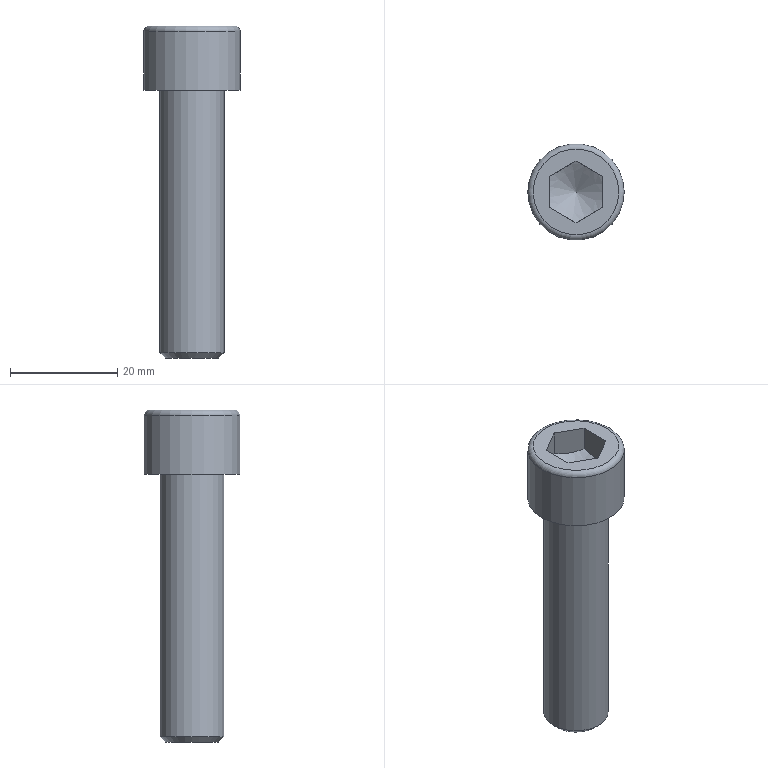Part | NX | features solid 2 | 1 solid | 14 faces | box 18 x 18 x 62 mm | volume 8162 mm3 | plane 9 | cylinder 2 | cone 2 | torus 1 | commonest cylinder face diameters 12 x1 18 x1
STEP:
#1=CARTESIAN_POINT('',(243.,-220.,-80.));
#2=VERTEX_POINT('',#1);
#3=CARTESIAN_POINT('',(235.,-220.,-80.));
#4=DIRECTION('',(0.,0.,1.));
#5=DIRECTION('',(1.,0.,0.));
#6=AXIS2_PLACEMENT_3D('',#3,#4,#5);
#7=CIRCLE('',#6,8.);
#8=EDGE_CURVE('',#2,#2,#7,.T.);
#9=ORIENTED_EDGE('',*,*,#8,.T.);
#10=EDGE_LOOP('',(#9));
#11=FACE_BOUND('',#10,.T.);
#12=CARTESIAN_POINT('',(240.,-222.887,-80.));
#13=VERTEX_POINT('',#12);
#14=CARTESIAN_POINT('',(235.,-225.774,-80.));
#15=VERTEX_POINT('',#14);
#16=CARTESIAN_POINT('',(240.,-222.887,-80.));
#17=DIRECTION('',(-0.866,-0.5,0.));
#18=VECTOR('',#17,1000.);
#19=LINE('',#16,#18);
#20=EDGE_CURVE('',#13,#15,#19,.T.);
#21=ORIENTED_EDGE('',*,*,#20,.T.);
#22=CARTESIAN_POINT('',(230.,-222.887,-80.));
#23=VERTEX_POINT('',#22);
#24=CARTESIAN_POINT('',(235.,-225.774,-80.));
#25=DIRECTION('',(-0.866,0.5,0.));
#26=VECTOR('',#25,1000.);
#27=LINE('',#24,#26);
#28=EDGE_CURVE('',#15,#23,#27,.T.);
#29=ORIENTED_EDGE('',*,*,#28,.T.);
#30=CARTESIAN_POINT('',(230.,-217.113,-80.));
#31=VERTEX_POINT('',#30);
#32=CARTESIAN_POINT('',(230.,-222.887,-80.));
#33=DIRECTION('',(0.,1.,0.));
#34=VECTOR('',#33,1000.);
#35=LINE('',#32,#34);
#36=EDGE_CURVE('',#23,#31,#35,.T.);
#37=ORIENTED_EDGE('',*,*,#36,.T.);
#38=CARTESIAN_POINT('',(235.,-214.226,-80.));
#39=VERTEX_POINT('',#38);
#40=CARTESIAN_POINT('',(230.,-217.113,-80.));
#41=DIRECTION('',(0.866,0.5,0.));
#42=VECTOR('',#41,1000.);
#43=LINE('',#40,#42);
#44=EDGE_CURVE('',#31,#39,#43,.T.);
#45=ORIENTED_EDGE('',*,*,#44,.T.);
#46=CARTESIAN_POINT('',(240.,-217.113,-80.));
#47=VERTEX_POINT('',#46);
#48=CARTESIAN_POINT('',(235.,-214.226,-80.));
#49=DIRECTION('',(0.866,-0.5,0.));
#50=VECTOR('',#49,1000.);
#51=LINE('',#48,#50);
#52=EDGE_CURVE('',#39,#47,#51,.T.);
#53=ORIENTED_EDGE('',*,*,#52,.T.);
#54=CARTESIAN_POINT('',(240.,-217.113,-80.));
#55=DIRECTION('',(0.,-1.,0.));
#56=VECTOR('',#55,1000.);
#57=LINE('',#54,#56);
#58=EDGE_CURVE('',#47,#13,#57,.T.);
#59=ORIENTED_EDGE('',*,*,#58,.T.);
#60=EDGE_LOOP('',(#21,#29,#37,#45,#53,#59));
#61=FACE_BOUND('',#60,.T.);
#62=CARTESIAN_POINT('',(235.,-220.,-80.));
#63=DIRECTION('',(0.,0.,1.));
#64=DIRECTION('',(1.,0.,0.));
#65=AXIS2_PLACEMENT_3D('',#62,#63,#64);
#66=PLANE('',#65);
#67=ADVANCED_FACE('',(#11,#61),#66,.T.);
#68=CARTESIAN_POINT('',(229.,-220.,-92.));
#69=VERTEX_POINT('',#68);
#70=CARTESIAN_POINT('',(235.,-220.,-92.));
#71=DIRECTION('',(0.,0.,-1.));
#72=DIRECTION('',(-1.,0.,0.));
#73=AXIS2_PLACEMENT_3D('',#70,#71,#72);
#74=CIRCLE('',#73,6.);
#75=EDGE_CURVE('',#69,#69,#74,.T.);
#76=ORIENTED_EDGE('',*,*,#75,.F.);
#77=EDGE_LOOP('',(#76));
#78=FACE_BOUND('',#77,.T.);
#79=CARTESIAN_POINT('',(244.,-220.,-92.));
#80=VERTEX_POINT('',#79);
#81=CARTESIAN_POINT('',(235.,-220.,-92.));
#82=DIRECTION('',(0.,0.,1.));
#83=DIRECTION('',(1.,0.,0.));
#84=AXIS2_PLACEMENT_3D('',#81,#82,#83);
#85=CIRCLE('',#84,9.);
#86=EDGE_CURVE('',#80,#80,#85,.T.);
#87=ORIENTED_EDGE('',*,*,#86,.F.);
#88=EDGE_LOOP('',(#87));
#89=FACE_BOUND('',#88,.T.);
#90=CARTESIAN_POINT('',(235.,-220.,-92.));
#91=DIRECTION('',(0.,0.,-1.));
#92=DIRECTION('',(-1.,0.,0.));
#93=AXIS2_PLACEMENT_3D('',#90,#91,#92);
#94=PLANE('',#93);
#95=ADVANCED_FACE('',(#78,#89),#94,.T.);
#96=CARTESIAN_POINT('',(244.,-220.,-81.));
#97=VERTEX_POINT('',#96);
#98=CARTESIAN_POINT('',(235.,-220.,-81.));
#99=DIRECTION('',(0.,0.,1.));
#100=DIRECTION('',(1.,0.,0.));
#101=AXIS2_PLACEMENT_3D('',#98,#99,#100);
#102=CIRCLE('',#101,9.);
#103=EDGE_CURVE('',#97,#97,#102,.F.);
#104=ORIENTED_EDGE('',*,*,#103,.T.);
#105=EDGE_LOOP('',(#104));
#106=FACE_BOUND('',#105,.T.);
#107=ORIENTED_EDGE('',*,*,#86,.T.);
#108=EDGE_LOOP('',(#107));
#109=FACE_BOUND('',#108,.T.);
#110=CARTESIAN_POINT('',(235.,-220.,-92.));
#111=DIRECTION('',(0.,0.,1.));
#112=DIRECTION('',(1.,0.,0.));
#113=AXIS2_PLACEMENT_3D('',#110,#111,#112);
#114=CYLINDRICAL_SURFACE('',#113,9.);
#115=ADVANCED_FACE('',(#106,#109),#114,.T.);
#116=CARTESIAN_POINT('',(235.,-225.774,-84.667));
#117=VERTEX_POINT('',#116);
#118=CARTESIAN_POINT('',(235.,-225.774,-80.));
#119=DIRECTION('',(0.,0.,-1.));
#120=VECTOR('',#119,1000.);
#121=LINE('',#118,#120);
#122=EDGE_CURVE('',#15,#117,#121,.T.);
#123=ORIENTED_EDGE('',*,*,#122,.F.);
#124=ORIENTED_EDGE('',*,*,#20,.F.);
#125=CARTESIAN_POINT('',(240.,-222.887,-84.667));
#126=VERTEX_POINT('',#125);
#127=CARTESIAN_POINT('',(240.,-222.887,-80.));
#128=DIRECTION('',(0.,0.,-1.));
#129=VECTOR('',#128,1000.);
#130=LINE('',#127,#129);
#131=EDGE_CURVE('',#13,#126,#130,.T.);
#132=ORIENTED_EDGE('',*,*,#131,.T.);
#133=CARTESIAN_POINT('',(235.,-225.774,-84.667));
#134=CARTESIAN_POINT('',(235.816,-225.302,-84.939));
#135=CARTESIAN_POINT('',(237.491,-224.335,-85.288));
#136=CARTESIAN_POINT('',(239.183,-223.359,-84.939));
#137=CARTESIAN_POINT('',(240.,-222.887,-84.667));
#138=B_SPLINE_CURVE_WITH_KNOTS('',3,(#133,#134,#135,#136,#137),.UNSPECIFIED.,.F.,.F.,(4,1,4),(0.000000238,0.002916,0.005831),.UNSPECIFIED.);
#139=EDGE_CURVE('',#117,#126,#138,.T.);
#140=ORIENTED_EDGE('',*,*,#139,.F.);
#141=EDGE_LOOP('',(#123,#124,#132,#140));
#142=FACE_BOUND('',#141,.T.);
#143=CARTESIAN_POINT('',(237.5,-224.33,-84.));
#144=DIRECTION('',(0.5,-0.866,0.));
#145=DIRECTION('',(0.866,0.5,0.));
#146=AXIS2_PLACEMENT_3D('',#143,#144,#145);
#147=PLANE('',#146);
#148=ADVANCED_FACE('',(#142),#147,.F.);
#149=ORIENTED_EDGE('',*,*,#131,.F.);
#150=ORIENTED_EDGE('',*,*,#58,.F.);
#151=CARTESIAN_POINT('',(240.,-217.113,-84.667));
#152=VERTEX_POINT('',#151);
#153=CARTESIAN_POINT('',(240.,-217.113,-80.));
#154=DIRECTION('',(0.,0.,-1.));
#155=VECTOR('',#154,1000.);
#156=LINE('',#153,#155);
#157=EDGE_CURVE('',#47,#152,#156,.T.);
#158=ORIENTED_EDGE('',*,*,#157,.T.);
#159=CARTESIAN_POINT('',(240.,-222.887,-84.667));
#160=CARTESIAN_POINT('',(240.,-221.948,-84.938));
#161=CARTESIAN_POINT('',(240.,-220.001,-85.29));
#162=CARTESIAN_POINT('',(240.,-218.046,-84.936));
#163=CARTESIAN_POINT('',(240.,-217.113,-84.667));
#164=B_SPLINE_CURVE_WITH_KNOTS('',3,(#159,#160,#161,#162,#163),.UNSPECIFIED.,.F.,.F.,(4,1,4),(0.005117,0.008037,0.01096),.UNSPECIFIED.);
#165=EDGE_CURVE('',#126,#152,#164,.T.);
#166=ORIENTED_EDGE('',*,*,#165,.F.);
#167=EDGE_LOOP('',(#149,#150,#158,#166));
#168=FACE_BOUND('',#167,.T.);
#169=CARTESIAN_POINT('',(240.,-220.,-84.));
#170=DIRECTION('',(1.,0.,0.));
#171=DIRECTION('',(0.,0.,-1.));
#172=AXIS2_PLACEMENT_3D('',#169,#170,#171);
#173=PLANE('',#172);
#174=ADVANCED_FACE('',(#168),#173,.F.);
#175=ORIENTED_EDGE('',*,*,#157,.F.);
#176=ORIENTED_EDGE('',*,*,#52,.F.);
#177=CARTESIAN_POINT('',(235.,-214.226,-84.667));
#178=VERTEX_POINT('',#177);
#179=CARTESIAN_POINT('',(235.,-214.226,-80.));
#180=DIRECTION('',(0.,0.,-1.));
#181=VECTOR('',#180,1000.);
#182=LINE('',#179,#181);
#183=EDGE_CURVE('',#39,#178,#182,.T.);
#184=ORIENTED_EDGE('',*,*,#183,.T.);
#185=CARTESIAN_POINT('',(240.,-217.113,-84.667));
#186=CARTESIAN_POINT('',(239.184,-216.642,-84.939));
#187=CARTESIAN_POINT('',(237.509,-215.675,-85.288));
#188=CARTESIAN_POINT('',(235.817,-214.698,-84.939));
#189=CARTESIAN_POINT('',(235.,-214.226,-84.667));
#190=B_SPLINE_CURVE_WITH_KNOTS('',3,(#185,#186,#187,#188,#189),.UNSPECIFIED.,.F.,.F.,(4,1,4),(0.000000238,0.002916,0.005831),.UNSPECIFIED.);
#191=EDGE_CURVE('',#152,#178,#190,.T.);
#192=ORIENTED_EDGE('',*,*,#191,.F.);
#193=EDGE_LOOP('',(#175,#176,#184,#192));
#194=FACE_BOUND('',#193,.T.);
#195=CARTESIAN_POINT('',(237.5,-215.67,-84.));
#196=DIRECTION('',(0.5,0.866,0.));
#197=DIRECTION('',(-0.866,0.5,0.));
#198=AXIS2_PLACEMENT_3D('',#195,#196,#197);
#199=PLANE('',#198);
#200=ADVANCED_FACE('',(#194),#199,.F.);
#201=ORIENTED_EDGE('',*,*,#183,.F.);
#202=ORIENTED_EDGE('',*,*,#44,.F.);
#203=CARTESIAN_POINT('',(230.,-217.113,-84.667));
#204=VERTEX_POINT('',#203);
#205=CARTESIAN_POINT('',(230.,-217.113,-80.));
#206=DIRECTION('',(0.,0.,-1.));
#207=VECTOR('',#206,1000.);
#208=LINE('',#205,#207);
#209=EDGE_CURVE('',#31,#204,#208,.T.);
#210=ORIENTED_EDGE('',*,*,#209,.T.);
#211=CARTESIAN_POINT('',(235.,-214.226,-84.667));
#212=CARTESIAN_POINT('',(234.184,-214.698,-84.939));
#213=CARTESIAN_POINT('',(232.509,-215.665,-85.288));
#214=CARTESIAN_POINT('',(230.817,-216.641,-84.939));
#215=CARTESIAN_POINT('',(230.,-217.113,-84.667));
#216=B_SPLINE_CURVE_WITH_KNOTS('',3,(#211,#212,#213,#214,#215),.UNSPECIFIED.,.F.,.F.,(4,1,4),(0.000000238,0.002916,0.005831),.UNSPECIFIED.);
#217=EDGE_CURVE('',#178,#204,#216,.T.);
#218=ORIENTED_EDGE('',*,*,#217,.F.);
#219=EDGE_LOOP('',(#201,#202,#210,#218));
#220=FACE_BOUND('',#219,.T.);
#221=CARTESIAN_POINT('',(232.5,-215.67,-84.));
#222=DIRECTION('',(-0.5,0.866,0.));
#223=DIRECTION('',(-0.866,-0.5,0.));
#224=AXIS2_PLACEMENT_3D('',#221,#222,#223);
#225=PLANE('',#224);
#226=ADVANCED_FACE('',(#220),#225,.F.);
#227=ORIENTED_EDGE('',*,*,#209,.F.);
#228=ORIENTED_EDGE('',*,*,#36,.F.);
#229=CARTESIAN_POINT('',(230.,-222.887,-84.667));
#230=VERTEX_POINT('',#229);
#231=CARTESIAN_POINT('',(230.,-222.887,-80.));
#232=DIRECTION('',(0.,0.,-1.));
#233=VECTOR('',#232,1000.);
#234=LINE('',#231,#233);
#235=EDGE_CURVE('',#23,#230,#234,.T.);
#236=ORIENTED_EDGE('',*,*,#235,.T.);
#237=CARTESIAN_POINT('',(230.,-222.887,-84.667));
#238=CARTESIAN_POINT('',(230.,-221.948,-84.938));
#239=CARTESIAN_POINT('',(230.,-220.001,-85.29));
#240=CARTESIAN_POINT('',(230.,-218.046,-84.936));
#241=CARTESIAN_POINT('',(230.,-217.113,-84.667));
#242=B_SPLINE_CURVE_WITH_KNOTS('',3,(#237,#238,#239,#240,#241),.UNSPECIFIED.,.F.,.F.,(4,1,4),(0.005117,0.008037,0.01096),.UNSPECIFIED.);
#243=EDGE_CURVE('',#204,#230,#242,.F.);
#244=ORIENTED_EDGE('',*,*,#243,.F.);
#245=EDGE_LOOP('',(#227,#228,#236,#244));
#246=FACE_BOUND('',#245,.T.);
#247=CARTESIAN_POINT('',(230.,-220.,-84.));
#248=DIRECTION('',(-1.,0.,0.));
#249=DIRECTION('',(0.,0.,1.));
#250=AXIS2_PLACEMENT_3D('',#247,#248,#249);
#251=PLANE('',#250);
#252=ADVANCED_FACE('',(#246),#251,.F.);
#253=ORIENTED_EDGE('',*,*,#235,.F.);
#254=ORIENTED_EDGE('',*,*,#28,.F.);
#255=ORIENTED_EDGE('',*,*,#122,.T.);
#256=CARTESIAN_POINT('',(230.,-222.887,-84.667));
#257=CARTESIAN_POINT('',(230.816,-223.358,-84.939));
#258=CARTESIAN_POINT('',(232.491,-224.325,-85.288));
#259=CARTESIAN_POINT('',(234.183,-225.302,-84.939));
#260=CARTESIAN_POINT('',(235.,-225.774,-84.667));
#261=B_SPLINE_CURVE_WITH_KNOTS('',3,(#256,#257,#258,#259,#260),.UNSPECIFIED.,.F.,.F.,(4,1,4),(0.000000238,0.002916,0.005831),.UNSPECIFIED.);
#262=EDGE_CURVE('',#230,#117,#261,.T.);
#263=ORIENTED_EDGE('',*,*,#262,.F.);
#264=EDGE_LOOP('',(#253,#254,#255,#263));
#265=FACE_BOUND('',#264,.T.);
#266=CARTESIAN_POINT('',(232.5,-224.33,-84.));
#267=DIRECTION('',(-0.5,-0.866,0.));
#268=DIRECTION('',(0.866,-0.5,0.));
#269=AXIS2_PLACEMENT_3D('',#266,#267,#268);
#270=PLANE('',#269);
#271=ADVANCED_FACE('',(#265),#270,.F.);
#272=ORIENTED_EDGE('',*,*,#139,.T.);
#273=ORIENTED_EDGE('',*,*,#165,.T.);
#274=ORIENTED_EDGE('',*,*,#191,.T.);
#275=ORIENTED_EDGE('',*,*,#217,.T.);
#276=ORIENTED_EDGE('',*,*,#243,.T.);
#277=ORIENTED_EDGE('',*,*,#262,.T.);
#278=EDGE_LOOP('',(#272,#273,#274,#275,#276,#277));
#279=FACE_BOUND('',#278,.T.);
#280=CARTESIAN_POINT('',(235.,-220.,-88.));
#281=VERTEX_POINT('',#280);
#282=VERTEX_LOOP('',#281);
#283=FACE_BOUND('',#282,.T.);
#284=CARTESIAN_POINT('',(235.,-220.,-88.));
#285=DIRECTION('',(0.,0.,1.));
#286=DIRECTION('',(1.,0.,0.));
#287=AXIS2_PLACEMENT_3D('',#284,#285,#286);
#288=CONICAL_SURFACE('',#287,0.,1.047);
#289=ADVANCED_FACE('',(#279,#283),#288,.F.);
#290=ORIENTED_EDGE('',*,*,#8,.F.);
#291=EDGE_LOOP('',(#290));
#292=FACE_BOUND('',#291,.T.);
#293=ORIENTED_EDGE('',*,*,#103,.F.);
#294=EDGE_LOOP('',(#293));
#295=FACE_BOUND('',#294,.T.);
#296=CARTESIAN_POINT('',(235.,-220.,-81.));
#297=DIRECTION('',(0.,0.,1.));
#298=DIRECTION('',(1.,0.,0.));
#299=AXIS2_PLACEMENT_3D('',#296,#297,#298);
#300=TOROIDAL_SURFACE('',#299,8.,1.);
#301=ADVANCED_FACE('',(#292,#295),#300,.T.);
#302=CARTESIAN_POINT('',(230.,-220.,-142.));
#303=VERTEX_POINT('',#302);
#304=CARTESIAN_POINT('',(235.,-220.,-142.));
#305=DIRECTION('',(0.,0.,-1.));
#306=DIRECTION('',(-1.,0.,0.));
#307=AXIS2_PLACEMENT_3D('',#304,#305,#306);
#308=CIRCLE('',#307,5.);
#309=EDGE_CURVE('',#303,#303,#308,.T.);
#310=ORIENTED_EDGE('',*,*,#309,.T.);
#311=EDGE_LOOP('',(#310));
#312=FACE_BOUND('',#311,.T.);
#313=CARTESIAN_POINT('',(235.,-220.,-142.));
#314=DIRECTION('',(0.,0.,-1.));
#315=DIRECTION('',(-1.,0.,0.));
#316=AXIS2_PLACEMENT_3D('',#313,#314,#315);
#317=PLANE('',#316);
#318=ADVANCED_FACE('',(#312),#317,.T.);
#319=CARTESIAN_POINT('',(229.,-220.,-141.));
#320=VERTEX_POINT('',#319);
#321=CARTESIAN_POINT('',(235.,-220.,-141.));
#322=DIRECTION('',(0.,0.,-1.));
#323=DIRECTION('',(-1.,0.,0.));
#324=AXIS2_PLACEMENT_3D('',#321,#322,#323);
#325=CIRCLE('',#324,6.);
#326=EDGE_CURVE('',#320,#320,#325,.F.);
#327=ORIENTED_EDGE('',*,*,#326,.T.);
#328=EDGE_LOOP('',(#327));
#329=FACE_BOUND('',#328,.T.);
#330=ORIENTED_EDGE('',*,*,#75,.T.);
#331=EDGE_LOOP('',(#330));
#332=FACE_BOUND('',#331,.T.);
#333=CARTESIAN_POINT('',(235.,-220.,-92.));
#334=DIRECTION('',(0.,0.,-1.));
#335=DIRECTION('',(-1.,0.,0.));
#336=AXIS2_PLACEMENT_3D('',#333,#334,#335);
#337=CYLINDRICAL_SURFACE('',#336,6.);
#338=ADVANCED_FACE('',(#329,#332),#337,.T.);
#339=ORIENTED_EDGE('',*,*,#309,.F.);
#340=EDGE_LOOP('',(#339));
#341=FACE_BOUND('',#340,.T.);
#342=ORIENTED_EDGE('',*,*,#326,.F.);
#343=EDGE_LOOP('',(#342));
#344=FACE_BOUND('',#343,.T.);
#345=CARTESIAN_POINT('',(235.,-220.,-141.));
#346=DIRECTION('',(0.,0.,1.));
#347=DIRECTION('',(1.,0.,0.));
#348=AXIS2_PLACEMENT_3D('',#345,#346,#347);
#349=CONICAL_SURFACE('',#348,6.,0.7854);
#350=ADVANCED_FACE('',(#341,#344),#349,.T.);
#351=CLOSED_SHELL('',(#67,#95,#115,#148,#174,#200,#226,#252,#271,#289,#301,#318,#338,#350));
#352=MANIFOLD_SOLID_BREP('',#351);
#353=(LENGTH_UNIT()NAMED_UNIT(*)SI_UNIT(.MILLI.,.METRE.));
#354=UNCERTAINTY_MEASURE_WITH_UNIT(LENGTH_MEASURE(0.0508),#353,'','');
#355=(NAMED_UNIT(*)PLANE_ANGLE_UNIT()SI_UNIT($,.RADIAN.));
#356=(NAMED_UNIT(*)SI_UNIT($,.STERADIAN.)SOLID_ANGLE_UNIT());
#357=(GEOMETRIC_REPRESENTATION_CONTEXT(3)GLOBAL_UNCERTAINTY_ASSIGNED_CONTEXT((#354))GLOBAL_UNIT_ASSIGNED_CONTEXT((#353,#355,#356))REPRESENTATION_CONTEXT('',''));
#358=ADVANCED_BREP_SHAPE_REPRESENTATION('',(#352),#357);